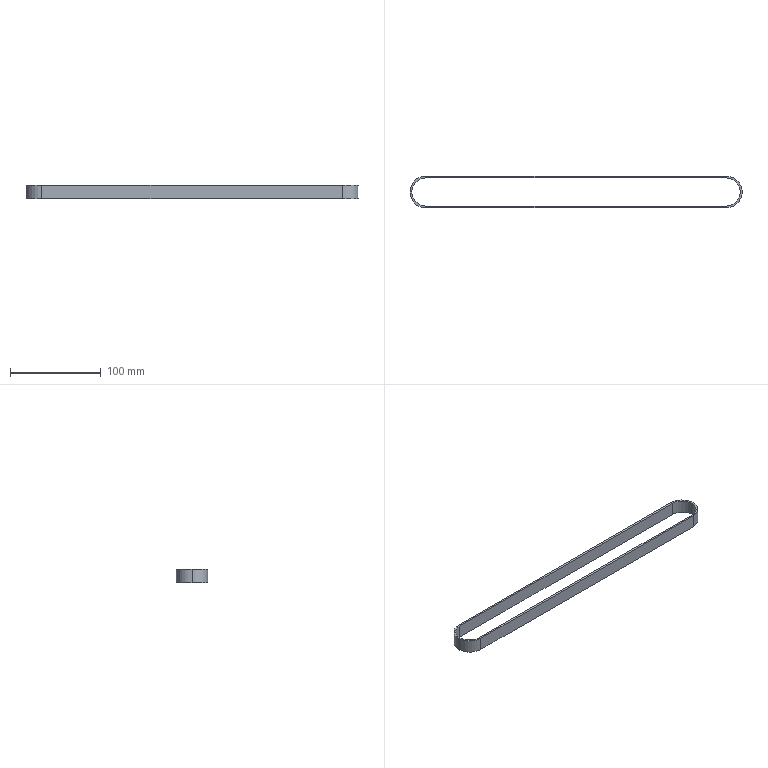Part | SolidWorks | features BaseBody 1 | 1 solid | 12 faces | box 365.37 x 34.87 x 15 mm | volume 22928 mm3 | plane 6 | cylinder 6 | commonest cylinder face diameters 30.87 x3 34.87 x3
STEP:
#1=CARTESIAN_POINT('',(-330.5,-15.435,-7.5));
#2=VERTEX_POINT('',#1);
#3=CARTESIAN_POINT('',(0.,-15.435,-7.5));
#4=VERTEX_POINT('',#3);
#5=CARTESIAN_POINT('',(0.,-15.435,-7.5));
#6=DIRECTION('',(1.,0.,0.));
#7=VECTOR('',#6,1000.);
#8=LINE('',#5,#7);
#9=EDGE_CURVE('',#2,#4,#8,.T.);
#10=ORIENTED_EDGE('',*,*,#9,.F.);
#11=CARTESIAN_POINT('',(-330.5,-15.435,7.5));
#12=VERTEX_POINT('',#11);
#13=CARTESIAN_POINT('',(-330.5,-15.435,7.5));
#14=DIRECTION('',(0.,0.,-1.));
#15=VECTOR('',#14,1000.);
#16=LINE('',#13,#15);
#17=EDGE_CURVE('',#12,#2,#16,.T.);
#18=ORIENTED_EDGE('',*,*,#17,.F.);
#19=CARTESIAN_POINT('',(0.,-15.435,7.5));
#20=VERTEX_POINT('',#19);
#21=CARTESIAN_POINT('',(0.,-15.435,7.5));
#22=DIRECTION('',(1.,0.,0.));
#23=VECTOR('',#22,1000.);
#24=LINE('',#21,#23);
#25=EDGE_CURVE('',#12,#20,#24,.T.);
#26=ORIENTED_EDGE('',*,*,#25,.T.);
#27=CARTESIAN_POINT('',(0.,-15.435,7.5));
#28=DIRECTION('',(0.,0.,-1.));
#29=VECTOR('',#28,1000.);
#30=LINE('',#27,#29);
#31=EDGE_CURVE('',#20,#4,#30,.T.);
#32=ORIENTED_EDGE('',*,*,#31,.T.);
#33=EDGE_LOOP('',(#10,#18,#26,#32));
#34=FACE_OUTER_BOUND('',#33,.T.);
#35=CARTESIAN_POINT('',(0.,-15.435,7.5));
#36=DIRECTION('',(0.,1.,0.));
#37=DIRECTION('',(1.,0.,0.));
#38=AXIS2_PLACEMENT_3D('',#35,#36,#37);
#39=PLANE('',#38);
#40=ADVANCED_FACE('',(#34),#39,.T.);
#41=CARTESIAN_POINT('',(-345.935,0.,7.5));
#42=VERTEX_POINT('',#41);
#43=CARTESIAN_POINT('',(-345.935,0.,-7.5));
#44=VERTEX_POINT('',#43);
#45=CARTESIAN_POINT('',(-345.935,0.,7.5));
#46=DIRECTION('',(0.,0.,-1.));
#47=VECTOR('',#46,1000.);
#48=LINE('',#45,#47);
#49=EDGE_CURVE('',#42,#44,#48,.T.);
#50=ORIENTED_EDGE('',*,*,#49,.F.);
#51=CARTESIAN_POINT('',(-330.5,0.,7.5));
#52=DIRECTION('',(0.,0.,1.));
#53=DIRECTION('',(-1.,0.,0.));
#54=AXIS2_PLACEMENT_3D('',#51,#52,#53);
#55=CIRCLE('',#54,15.435);
#56=EDGE_CURVE('',#42,#12,#55,.T.);
#57=ORIENTED_EDGE('',*,*,#56,.T.);
#58=ORIENTED_EDGE('',*,*,#17,.T.);
#59=CARTESIAN_POINT('',(-330.5,0.,-7.5));
#60=DIRECTION('',(0.,0.,1.));
#61=DIRECTION('',(-1.,0.,0.));
#62=AXIS2_PLACEMENT_3D('',#59,#60,#61);
#63=CIRCLE('',#62,15.435);
#64=EDGE_CURVE('',#44,#2,#63,.T.);
#65=ORIENTED_EDGE('',*,*,#64,.F.);
#66=EDGE_LOOP('',(#50,#57,#58,#65));
#67=FACE_OUTER_BOUND('',#66,.T.);
#68=CARTESIAN_POINT('',(-330.5,0.,7.5));
#69=DIRECTION('',(0.,0.,-1.));
#70=DIRECTION('',(-1.,0.,0.));
#71=AXIS2_PLACEMENT_3D('',#68,#69,#70);
#72=CYLINDRICAL_SURFACE('',#71,15.435);
#73=ADVANCED_FACE('',(#67),#72,.F.);
#74=CARTESIAN_POINT('',(0.,15.435,-7.5));
#75=VERTEX_POINT('',#74);
#76=CARTESIAN_POINT('',(-330.5,15.435,-7.5));
#77=VERTEX_POINT('',#76);
#78=CARTESIAN_POINT('',(-330.5,15.435,-7.5));
#79=DIRECTION('',(-1.,0.,0.));
#80=VECTOR('',#79,1000.);
#81=LINE('',#78,#80);
#82=EDGE_CURVE('',#75,#77,#81,.T.);
#83=ORIENTED_EDGE('',*,*,#82,.F.);
#84=CARTESIAN_POINT('',(0.,15.435,7.5));
#85=VERTEX_POINT('',#84);
#86=CARTESIAN_POINT('',(0.,15.435,7.5));
#87=DIRECTION('',(0.,0.,-1.));
#88=VECTOR('',#87,1000.);
#89=LINE('',#86,#88);
#90=EDGE_CURVE('',#85,#75,#89,.T.);
#91=ORIENTED_EDGE('',*,*,#90,.F.);
#92=CARTESIAN_POINT('',(-330.5,15.435,7.5));
#93=VERTEX_POINT('',#92);
#94=CARTESIAN_POINT('',(-330.5,15.435,7.5));
#95=DIRECTION('',(-1.,0.,0.));
#96=VECTOR('',#95,1000.);
#97=LINE('',#94,#96);
#98=EDGE_CURVE('',#85,#93,#97,.T.);
#99=ORIENTED_EDGE('',*,*,#98,.T.);
#100=CARTESIAN_POINT('',(-330.5,15.435,7.5));
#101=DIRECTION('',(0.,0.,-1.));
#102=VECTOR('',#101,1000.);
#103=LINE('',#100,#102);
#104=EDGE_CURVE('',#93,#77,#103,.T.);
#105=ORIENTED_EDGE('',*,*,#104,.T.);
#106=EDGE_LOOP('',(#83,#91,#99,#105));
#107=FACE_OUTER_BOUND('',#106,.T.);
#108=CARTESIAN_POINT('',(-330.5,15.435,7.5));
#109=DIRECTION('',(0.,-1.,0.));
#110=DIRECTION('',(0.,0.,-1.));
#111=AXIS2_PLACEMENT_3D('',#108,#109,#110);
#112=PLANE('',#111);
#113=ADVANCED_FACE('',(#107),#112,.T.);
#114=CARTESIAN_POINT('',(0.,0.,-7.5));
#115=DIRECTION('',(0.,0.,1.));
#116=DIRECTION('',(-1.,0.,0.));
#117=AXIS2_PLACEMENT_3D('',#114,#115,#116);
#118=CIRCLE('',#117,15.435);
#119=EDGE_CURVE('',#4,#75,#118,.T.);
#120=ORIENTED_EDGE('',*,*,#119,.F.);
#121=ORIENTED_EDGE('',*,*,#31,.F.);
#122=CARTESIAN_POINT('',(0.,0.,7.5));
#123=DIRECTION('',(0.,0.,1.));
#124=DIRECTION('',(-1.,0.,0.));
#125=AXIS2_PLACEMENT_3D('',#122,#123,#124);
#126=CIRCLE('',#125,15.435);
#127=EDGE_CURVE('',#20,#85,#126,.T.);
#128=ORIENTED_EDGE('',*,*,#127,.T.);
#129=ORIENTED_EDGE('',*,*,#90,.T.);
#130=EDGE_LOOP('',(#120,#121,#128,#129));
#131=FACE_OUTER_BOUND('',#130,.T.);
#132=CARTESIAN_POINT('',(0.,0.,7.5));
#133=DIRECTION('',(0.,0.,-1.));
#134=DIRECTION('',(-1.,0.,0.));
#135=AXIS2_PLACEMENT_3D('',#132,#133,#134);
#136=CYLINDRICAL_SURFACE('',#135,15.435);
#137=ADVANCED_FACE('',(#131),#136,.F.);
#138=CARTESIAN_POINT('',(-330.5,-17.435,-7.5));
#139=VERTEX_POINT('',#138);
#140=CARTESIAN_POINT('',(0.,-17.435,-7.5));
#141=VERTEX_POINT('',#140);
#142=CARTESIAN_POINT('',(0.,-17.435,-7.5));
#143=DIRECTION('',(1.,0.,0.));
#144=VECTOR('',#143,1000.);
#145=LINE('',#142,#144);
#146=EDGE_CURVE('',#139,#141,#145,.T.);
#147=ORIENTED_EDGE('',*,*,#146,.T.);
#148=CARTESIAN_POINT('',(0.,-17.435,7.5));
#149=VERTEX_POINT('',#148);
#150=CARTESIAN_POINT('',(0.,-17.435,7.5));
#151=DIRECTION('',(0.,0.,-1.));
#152=VECTOR('',#151,1000.);
#153=LINE('',#150,#152);
#154=EDGE_CURVE('',#149,#141,#153,.T.);
#155=ORIENTED_EDGE('',*,*,#154,.F.);
#156=CARTESIAN_POINT('',(-330.5,-17.435,7.5));
#157=VERTEX_POINT('',#156);
#158=CARTESIAN_POINT('',(0.,-17.435,7.5));
#159=DIRECTION('',(1.,0.,0.));
#160=VECTOR('',#159,1000.);
#161=LINE('',#158,#160);
#162=EDGE_CURVE('',#157,#149,#161,.T.);
#163=ORIENTED_EDGE('',*,*,#162,.F.);
#164=CARTESIAN_POINT('',(-330.5,-17.435,7.5));
#165=DIRECTION('',(0.,0.,-1.));
#166=VECTOR('',#165,1000.);
#167=LINE('',#164,#166);
#168=EDGE_CURVE('',#157,#139,#167,.T.);
#169=ORIENTED_EDGE('',*,*,#168,.T.);
#170=EDGE_LOOP('',(#147,#155,#163,#169));
#171=FACE_OUTER_BOUND('',#170,.T.);
#172=CARTESIAN_POINT('',(0.,-17.435,7.5));
#173=DIRECTION('',(0.,1.,0.));
#174=DIRECTION('',(1.,0.,0.));
#175=AXIS2_PLACEMENT_3D('',#172,#173,#174);
#176=PLANE('',#175);
#177=ADVANCED_FACE('',(#171),#176,.F.);
#178=CARTESIAN_POINT('',(-347.935,0.,7.5));
#179=VERTEX_POINT('',#178);
#180=CARTESIAN_POINT('',(-347.935,0.,-7.5));
#181=VERTEX_POINT('',#180);
#182=CARTESIAN_POINT('',(-347.935,0.,7.5));
#183=DIRECTION('',(0.,0.,-1.));
#184=VECTOR('',#183,1000.);
#185=LINE('',#182,#184);
#186=EDGE_CURVE('',#179,#181,#185,.T.);
#187=ORIENTED_EDGE('',*,*,#186,.F.);
#188=CARTESIAN_POINT('',(-330.5,17.435,7.5));
#189=VERTEX_POINT('',#188);
#190=CARTESIAN_POINT('',(-330.5,0.,7.5));
#191=DIRECTION('',(0.,0.,1.));
#192=DIRECTION('',(-1.,0.,0.));
#193=AXIS2_PLACEMENT_3D('',#190,#191,#192);
#194=CIRCLE('',#193,17.435);
#195=EDGE_CURVE('',#189,#179,#194,.T.);
#196=ORIENTED_EDGE('',*,*,#195,.F.);
#197=CARTESIAN_POINT('',(-330.5,17.435,-7.5));
#198=VERTEX_POINT('',#197);
#199=CARTESIAN_POINT('',(-330.5,17.435,7.5));
#200=DIRECTION('',(0.,0.,-1.));
#201=VECTOR('',#200,1000.);
#202=LINE('',#199,#201);
#203=EDGE_CURVE('',#189,#198,#202,.T.);
#204=ORIENTED_EDGE('',*,*,#203,.T.);
#205=CARTESIAN_POINT('',(-330.5,0.,-7.5));
#206=DIRECTION('',(0.,0.,1.));
#207=DIRECTION('',(-1.,0.,0.));
#208=AXIS2_PLACEMENT_3D('',#205,#206,#207);
#209=CIRCLE('',#208,17.435);
#210=EDGE_CURVE('',#198,#181,#209,.T.);
#211=ORIENTED_EDGE('',*,*,#210,.T.);
#212=EDGE_LOOP('',(#187,#196,#204,#211));
#213=FACE_OUTER_BOUND('',#212,.T.);
#214=CARTESIAN_POINT('',(-330.5,0.,7.5));
#215=DIRECTION('',(0.,0.,-1.));
#216=DIRECTION('',(-1.,0.,0.));
#217=AXIS2_PLACEMENT_3D('',#214,#215,#216);
#218=CYLINDRICAL_SURFACE('',#217,17.435);
#219=ADVANCED_FACE('',(#213),#218,.T.);
#220=CARTESIAN_POINT('',(0.,17.435,-7.5));
#221=VERTEX_POINT('',#220);
#222=CARTESIAN_POINT('',(0.,17.435,-7.5));
#223=DIRECTION('',(-1.,0.,0.));
#224=VECTOR('',#223,1000.);
#225=LINE('',#222,#224);
#226=EDGE_CURVE('',#221,#198,#225,.T.);
#227=ORIENTED_EDGE('',*,*,#226,.T.);
#228=ORIENTED_EDGE('',*,*,#203,.F.);
#229=CARTESIAN_POINT('',(0.,17.435,7.5));
#230=VERTEX_POINT('',#229);
#231=CARTESIAN_POINT('',(0.,17.435,7.5));
#232=DIRECTION('',(-1.,0.,0.));
#233=VECTOR('',#232,1000.);
#234=LINE('',#231,#233);
#235=EDGE_CURVE('',#230,#189,#234,.T.);
#236=ORIENTED_EDGE('',*,*,#235,.F.);
#237=CARTESIAN_POINT('',(0.,17.435,7.5));
#238=DIRECTION('',(0.,0.,-1.));
#239=VECTOR('',#238,1000.);
#240=LINE('',#237,#239);
#241=EDGE_CURVE('',#230,#221,#240,.T.);
#242=ORIENTED_EDGE('',*,*,#241,.T.);
#243=EDGE_LOOP('',(#227,#228,#236,#242));
#244=FACE_OUTER_BOUND('',#243,.T.);
#245=CARTESIAN_POINT('',(0.,17.435,7.5));
#246=DIRECTION('',(0.,-1.,0.));
#247=DIRECTION('',(0.,0.,-1.));
#248=AXIS2_PLACEMENT_3D('',#245,#246,#247);
#249=PLANE('',#248);
#250=ADVANCED_FACE('',(#244),#249,.F.);
#251=CARTESIAN_POINT('',(0.,0.,-7.5));
#252=DIRECTION('',(0.,0.,1.));
#253=DIRECTION('',(-1.,0.,0.));
#254=AXIS2_PLACEMENT_3D('',#251,#252,#253);
#255=CIRCLE('',#254,17.435);
#256=EDGE_CURVE('',#141,#221,#255,.T.);
#257=ORIENTED_EDGE('',*,*,#256,.T.);
#258=ORIENTED_EDGE('',*,*,#241,.F.);
#259=CARTESIAN_POINT('',(0.,0.,7.5));
#260=DIRECTION('',(0.,0.,1.));
#261=DIRECTION('',(-1.,0.,0.));
#262=AXIS2_PLACEMENT_3D('',#259,#260,#261);
#263=CIRCLE('',#262,17.435);
#264=EDGE_CURVE('',#149,#230,#263,.T.);
#265=ORIENTED_EDGE('',*,*,#264,.F.);
#266=ORIENTED_EDGE('',*,*,#154,.T.);
#267=EDGE_LOOP('',(#257,#258,#265,#266));
#268=FACE_OUTER_BOUND('',#267,.T.);
#269=CARTESIAN_POINT('',(0.,0.,7.5));
#270=DIRECTION('',(0.,0.,-1.));
#271=DIRECTION('',(-1.,0.,0.));
#272=AXIS2_PLACEMENT_3D('',#269,#270,#271);
#273=CYLINDRICAL_SURFACE('',#272,17.435);
#274=ADVANCED_FACE('',(#268),#273,.T.);
#275=ORIENTED_EDGE('',*,*,#9,.T.);
#276=ORIENTED_EDGE('',*,*,#119,.T.);
#277=ORIENTED_EDGE('',*,*,#82,.T.);
#278=CARTESIAN_POINT('',(-330.5,0.,-7.5));
#279=DIRECTION('',(0.,0.,1.));
#280=DIRECTION('',(-1.,0.,0.));
#281=AXIS2_PLACEMENT_3D('',#278,#279,#280);
#282=CIRCLE('',#281,15.435);
#283=EDGE_CURVE('',#77,#44,#282,.T.);
#284=ORIENTED_EDGE('',*,*,#283,.T.);
#285=ORIENTED_EDGE('',*,*,#64,.T.);
#286=EDGE_LOOP('',(#275,#276,#277,#284,#285));
#287=FACE_BOUND('',#286,.T.);
#288=ORIENTED_EDGE('',*,*,#256,.F.);
#289=ORIENTED_EDGE('',*,*,#146,.F.);
#290=CARTESIAN_POINT('',(-330.5,0.,-7.5));
#291=DIRECTION('',(0.,0.,1.));
#292=DIRECTION('',(-1.,0.,0.));
#293=AXIS2_PLACEMENT_3D('',#290,#291,#292);
#294=CIRCLE('',#293,17.435);
#295=EDGE_CURVE('',#181,#139,#294,.T.);
#296=ORIENTED_EDGE('',*,*,#295,.F.);
#297=ORIENTED_EDGE('',*,*,#210,.F.);
#298=ORIENTED_EDGE('',*,*,#226,.F.);
#299=EDGE_LOOP('',(#288,#289,#296,#297,#298));
#300=FACE_OUTER_BOUND('',#299,.T.);
#301=CARTESIAN_POINT('',(0.,0.,-7.5));
#302=DIRECTION('',(0.,0.,-1.));
#303=DIRECTION('',(0.,-1.,0.));
#304=AXIS2_PLACEMENT_3D('',#301,#302,#303);
#305=PLANE('',#304);
#306=ADVANCED_FACE('',(#287,#300),#305,.T.);
#307=ORIENTED_EDGE('',*,*,#127,.F.);
#308=ORIENTED_EDGE('',*,*,#25,.F.);
#309=ORIENTED_EDGE('',*,*,#56,.F.);
#310=CARTESIAN_POINT('',(-330.5,0.,7.5));
#311=DIRECTION('',(0.,0.,1.));
#312=DIRECTION('',(-1.,0.,0.));
#313=AXIS2_PLACEMENT_3D('',#310,#311,#312);
#314=CIRCLE('',#313,15.435);
#315=EDGE_CURVE('',#93,#42,#314,.T.);
#316=ORIENTED_EDGE('',*,*,#315,.F.);
#317=ORIENTED_EDGE('',*,*,#98,.F.);
#318=EDGE_LOOP('',(#307,#308,#309,#316,#317));
#319=FACE_BOUND('',#318,.T.);
#320=ORIENTED_EDGE('',*,*,#264,.T.);
#321=ORIENTED_EDGE('',*,*,#235,.T.);
#322=ORIENTED_EDGE('',*,*,#195,.T.);
#323=CARTESIAN_POINT('',(-330.5,0.,7.5));
#324=DIRECTION('',(0.,0.,1.));
#325=DIRECTION('',(-1.,0.,0.));
#326=AXIS2_PLACEMENT_3D('',#323,#324,#325);
#327=CIRCLE('',#326,17.435);
#328=EDGE_CURVE('',#179,#157,#327,.T.);
#329=ORIENTED_EDGE('',*,*,#328,.T.);
#330=ORIENTED_EDGE('',*,*,#162,.T.);
#331=EDGE_LOOP('',(#320,#321,#322,#329,#330));
#332=FACE_OUTER_BOUND('',#331,.T.);
#333=CARTESIAN_POINT('',(0.,0.,7.5));
#334=DIRECTION('',(0.,0.,-1.));
#335=DIRECTION('',(0.,-1.,0.));
#336=AXIS2_PLACEMENT_3D('',#333,#334,#335);
#337=PLANE('',#336);
#338=ADVANCED_FACE('',(#319,#332),#337,.F.);
#339=ORIENTED_EDGE('',*,*,#328,.F.);
#340=ORIENTED_EDGE('',*,*,#186,.T.);
#341=ORIENTED_EDGE('',*,*,#295,.T.);
#342=ORIENTED_EDGE('',*,*,#168,.F.);
#343=EDGE_LOOP('',(#339,#340,#341,#342));
#344=FACE_OUTER_BOUND('',#343,.T.);
#345=CARTESIAN_POINT('',(-330.5,0.,7.5));
#346=DIRECTION('',(0.,0.,-1.));
#347=DIRECTION('',(-1.,0.,0.));
#348=AXIS2_PLACEMENT_3D('',#345,#346,#347);
#349=CYLINDRICAL_SURFACE('',#348,17.435);
#350=ADVANCED_FACE('',(#344),#349,.T.);
#351=ORIENTED_EDGE('',*,*,#315,.T.);
#352=ORIENTED_EDGE('',*,*,#49,.T.);
#353=ORIENTED_EDGE('',*,*,#283,.F.);
#354=ORIENTED_EDGE('',*,*,#104,.F.);
#355=EDGE_LOOP('',(#351,#352,#353,#354));
#356=FACE_OUTER_BOUND('',#355,.T.);
#357=CARTESIAN_POINT('',(-330.5,0.,7.5));
#358=DIRECTION('',(0.,0.,-1.));
#359=DIRECTION('',(-1.,0.,0.));
#360=AXIS2_PLACEMENT_3D('',#357,#358,#359);
#361=CYLINDRICAL_SURFACE('',#360,15.435);
#362=ADVANCED_FACE('',(#356),#361,.F.);
#363=CLOSED_SHELL('',(#40,#73,#113,#137,#177,#219,#250,#274,#306,#338,#350,#362));
#364=MANIFOLD_SOLID_BREP('',#363);
#365=CARTESIAN_POINT('',(0.,0.,0.));
#366=DIRECTION('',(0.,0.,1.));
#367=DIRECTION('',(1.,0.,0.));
#368=AXIS2_PLACEMENT_3D('',#365,#366,#367);
#369=(LENGTH_UNIT()NAMED_UNIT(*)SI_UNIT(.MILLI.,.METRE.));
#370=UNCERTAINTY_MEASURE_WITH_UNIT(LENGTH_MEASURE(0.00001),#369,'','');
#371=(NAMED_UNIT(*)PLANE_ANGLE_UNIT()SI_UNIT($,.RADIAN.));
#372=(NAMED_UNIT(*)SI_UNIT($,.STERADIAN.)SOLID_ANGLE_UNIT());
#373=(GEOMETRIC_REPRESENTATION_CONTEXT(3)GLOBAL_UNCERTAINTY_ASSIGNED_CONTEXT((#370))GLOBAL_UNIT_ASSIGNED_CONTEXT((#369,#371,#372))REPRESENTATION_CONTEXT('',''));
#374=ADVANCED_BREP_SHAPE_REPRESENTATION('',(#364,#368),#373);